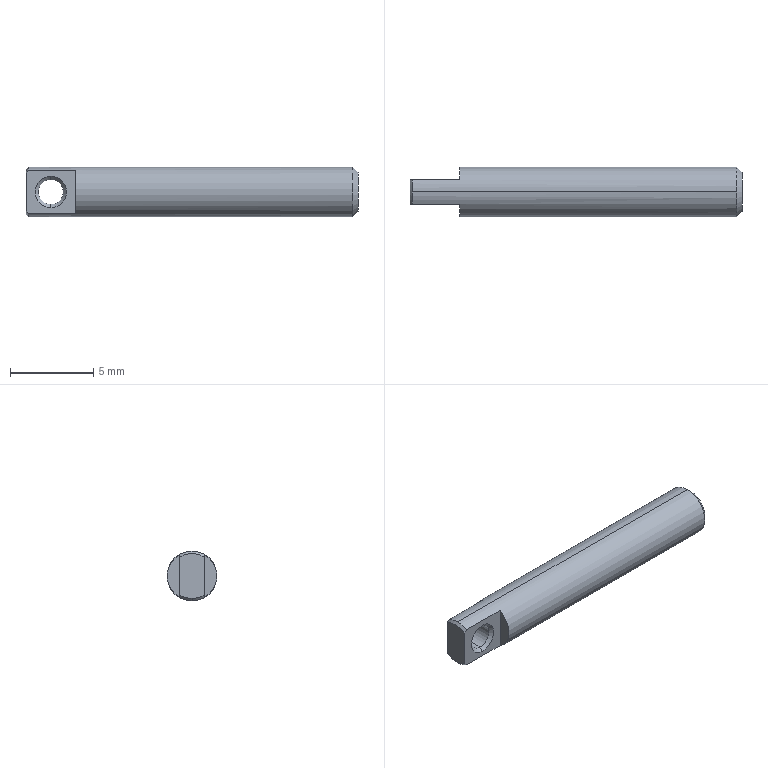Part | STEP file | 0246_Z_009_SAIPOZ3-20_1 | 1 solid | 19 faces | box 20 x 3 x 3 mm | volume 129.776 mm3 | cone 9 | plane 6 | cylinder 4 | commonest cylinder face diameters 1.5 x2 3 x2